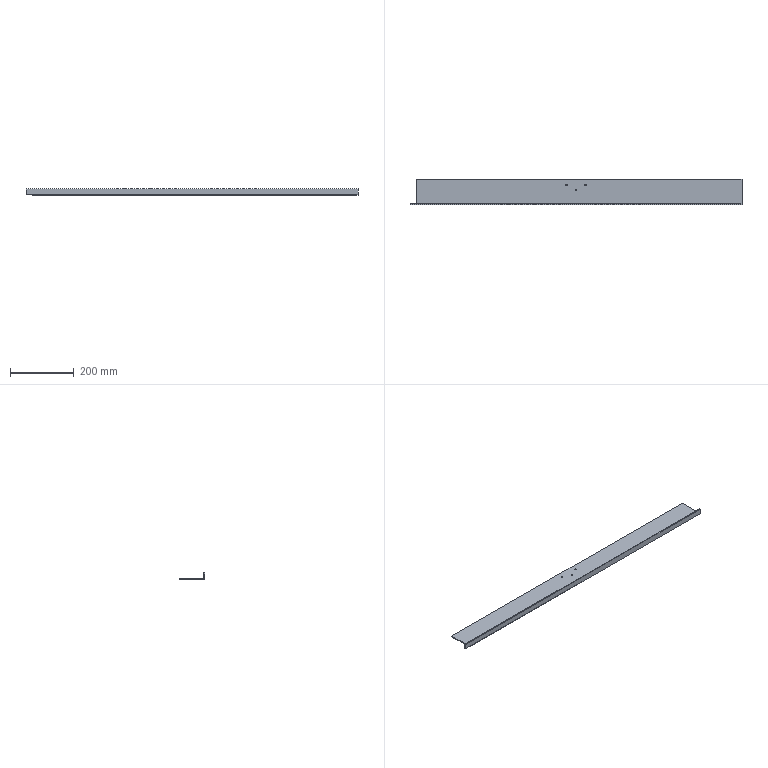Part | STEP file | HESS-408-70-15W-W-5-outer case reinforcing rib 1 | 1 solid | 19 faces | box 1043 x 80 x 20 mm | volume 296450 mm3 | plane 10 | cylinder 9 | commonest cylinder face diameters 4.2 x6 0.2 x1 2 x1 6.2 x1